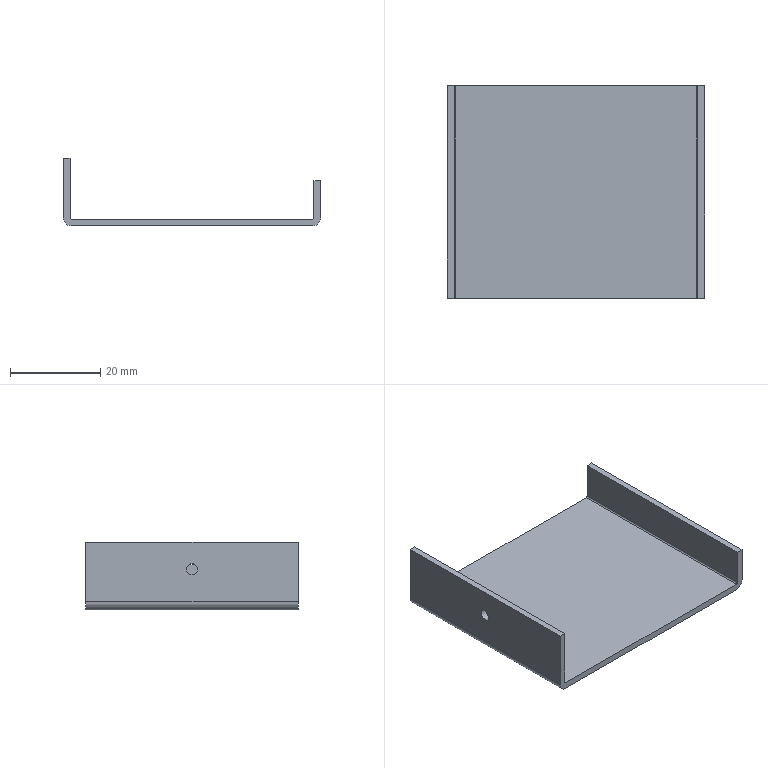Part | STEP file | FHD-021-008-01-B circuit breaker bracket 2 | 1 solid | 15 faces | box 57 x 47 x 15 mm | volume 5499 mm3 | plane 10 | cylinder 5 | commonest cylinder face diameters 0.6 x2 3.6 x2 2.5 x1
STEP:
#1=CARTESIAN_POINT('',(0.,0.,0.));
#2=DIRECTION('',(0.,0.,1.));
#3=DIRECTION('',(1.,0.,0.));
#4=AXIS2_PLACEMENT_3D('',#1,#2,#3);
#5=CARTESIAN_POINT('',(-26.7,23.5,-1.5));
#6=VERTEX_POINT('',#5);
#7=CARTESIAN_POINT('',(26.7,23.5,-1.5));
#8=VERTEX_POINT('',#7);
#9=CARTESIAN_POINT('',(0.,23.5,-1.5));
#10=DIRECTION('',(1.,0.,0.));
#11=VECTOR('',#10,1.);
#12=LINE('',#9,#11);
#13=CARTESIAN_POINT('',(0.,0.,-1.5));
#14=DIRECTION('',(0.,0.,-1.));
#15=DIRECTION('',(-1.,0.,0.));
#16=AXIS2_PLACEMENT_3D('',#13,#14,#15);
#17=PLANE('',#16);
#18=CARTESIAN_POINT('',(0.,23.5));
#19=DIRECTION('',(-1.,0.));
#20=VECTOR('',#19,1.);
#21=LINE('',#18,#20);
#22=(GEOMETRIC_REPRESENTATION_CONTEXT(2)PARAMETRIC_REPRESENTATION_CONTEXT()REPRESENTATION_CONTEXT('',''));
#23=DEFINITIONAL_REPRESENTATION('',(#21),#22);
#24=PCURVE('',#17,#23);
#25=CARTESIAN_POINT('',(-28.5,23.5,-1.5));
#26=DIRECTION('',(0.,1.,0.));
#27=DIRECTION('',(0.,0.,1.));
#28=AXIS2_PLACEMENT_3D('',#25,#26,#27);
#29=PLANE('',#28);
#30=CARTESIAN_POINT('',(0.,28.5));
#31=DIRECTION('',(0.,1.));
#32=VECTOR('',#31,1.);
#33=LINE('',#30,#32);
#34=(GEOMETRIC_REPRESENTATION_CONTEXT(2)PARAMETRIC_REPRESENTATION_CONTEXT()REPRESENTATION_CONTEXT('',''));
#35=DEFINITIONAL_REPRESENTATION('',(#33),#34);
#36=PCURVE('',#29,#35);
#37=SURFACE_CURVE('',#12,(#24,#36),.PCURVE_S1.);
#38=EDGE_CURVE('',#6,#8,#37,.T.);
#39=ORIENTED_EDGE('',*,*,#38,.T.);
#40=CARTESIAN_POINT('',(26.7,-23.5,-1.5));
#41=VERTEX_POINT('',#40);
#42=CARTESIAN_POINT('',(26.7,0.,-1.5));
#43=DIRECTION('',(0.,-1.,0.));
#44=VECTOR('',#43,1.);
#45=LINE('',#42,#44);
#46=CARTESIAN_POINT('',(-26.7,0.));
#47=DIRECTION('',(0.,-1.));
#48=VECTOR('',#47,1.);
#49=LINE('',#46,#48);
#50=(GEOMETRIC_REPRESENTATION_CONTEXT(2)PARAMETRIC_REPRESENTATION_CONTEXT()REPRESENTATION_CONTEXT('',''));
#51=DEFINITIONAL_REPRESENTATION('',(#49),#50);
#52=PCURVE('',#17,#51);
#53=CARTESIAN_POINT('',(26.7,23.5,0.3));
#54=DIRECTION('',(0.,1.,0.));
#55=DIRECTION('',(0.,0.,1.));
#56=AXIS2_PLACEMENT_3D('',#53,#54,#55);
#57=CYLINDRICAL_SURFACE('',#56,1.8);
#58=CARTESIAN_POINT('',(3.142,-23.5));
#59=DIRECTION('',(0.,-1.));
#60=VECTOR('',#59,1.);
#61=LINE('',#58,#60);
#62=(GEOMETRIC_REPRESENTATION_CONTEXT(2)PARAMETRIC_REPRESENTATION_CONTEXT()REPRESENTATION_CONTEXT('',''));
#63=DEFINITIONAL_REPRESENTATION('',(#61),#62);
#64=PCURVE('',#57,#63);
#65=SURFACE_CURVE('',#45,(#52,#64),.PCURVE_S1.);
#66=EDGE_CURVE('',#8,#41,#65,.T.);
#67=ORIENTED_EDGE('',*,*,#66,.T.);
#68=CARTESIAN_POINT('',(-26.7,-23.5,-1.5));
#69=VERTEX_POINT('',#68);
#70=CARTESIAN_POINT('',(0.,-23.5,-1.5));
#71=DIRECTION('',(-1.,0.,0.));
#72=VECTOR('',#71,1.);
#73=LINE('',#70,#72);
#74=CARTESIAN_POINT('',(0.,-23.5));
#75=DIRECTION('',(1.,0.));
#76=VECTOR('',#75,1.);
#77=LINE('',#74,#76);
#78=(GEOMETRIC_REPRESENTATION_CONTEXT(2)PARAMETRIC_REPRESENTATION_CONTEXT()REPRESENTATION_CONTEXT('',''));
#79=DEFINITIONAL_REPRESENTATION('',(#77),#78);
#80=PCURVE('',#17,#79);
#81=CARTESIAN_POINT('',(-28.5,-23.5,-1.5));
#82=DIRECTION('',(0.,-1.,0.));
#83=DIRECTION('',(0.,0.,-1.));
#84=AXIS2_PLACEMENT_3D('',#81,#82,#83);
#85=PLANE('',#84);
#86=CARTESIAN_POINT('',(0.,28.5));
#87=DIRECTION('',(0.,-1.));
#88=VECTOR('',#87,1.);
#89=LINE('',#86,#88);
#90=(GEOMETRIC_REPRESENTATION_CONTEXT(2)PARAMETRIC_REPRESENTATION_CONTEXT()REPRESENTATION_CONTEXT('',''));
#91=DEFINITIONAL_REPRESENTATION('',(#89),#90);
#92=PCURVE('',#85,#91);
#93=SURFACE_CURVE('',#73,(#80,#92),.PCURVE_S1.);
#94=EDGE_CURVE('',#41,#69,#93,.T.);
#95=ORIENTED_EDGE('',*,*,#94,.T.);
#96=CARTESIAN_POINT('',(-26.7,0.,-1.5));
#97=DIRECTION('',(0.,1.,0.));
#98=VECTOR('',#97,1.);
#99=LINE('',#96,#98);
#100=CARTESIAN_POINT('',(26.7,0.));
#101=DIRECTION('',(0.,1.));
#102=VECTOR('',#101,1.);
#103=LINE('',#100,#102);
#104=(GEOMETRIC_REPRESENTATION_CONTEXT(2)PARAMETRIC_REPRESENTATION_CONTEXT()REPRESENTATION_CONTEXT('',''));
#105=DEFINITIONAL_REPRESENTATION('',(#103),#104);
#106=PCURVE('',#17,#105);
#107=CARTESIAN_POINT('',(-26.7,-23.5,0.3));
#108=DIRECTION('',(0.,-1.,0.));
#109=DIRECTION('',(0.,0.,-1.));
#110=AXIS2_PLACEMENT_3D('',#107,#108,#109);
#111=CYLINDRICAL_SURFACE('',#110,1.8);
#112=CARTESIAN_POINT('',(6.283,-23.5));
#113=DIRECTION('',(0.,-1.));
#114=VECTOR('',#113,1.);
#115=LINE('',#112,#114);
#116=(GEOMETRIC_REPRESENTATION_CONTEXT(2)PARAMETRIC_REPRESENTATION_CONTEXT()REPRESENTATION_CONTEXT('',''));
#117=DEFINITIONAL_REPRESENTATION('',(#115),#116);
#118=PCURVE('',#111,#117);
#119=SURFACE_CURVE('',#99,(#106,#118),.PCURVE_S1.);
#120=EDGE_CURVE('',#69,#6,#119,.T.);
#121=ORIENTED_EDGE('',*,*,#120,.T.);
#122=EDGE_LOOP('',(#39,#67,#95,#121));
#123=FACE_BOUND('',#122,.T.);
#124=ADVANCED_FACE('',(#123),#17,.T.);
#125=CARTESIAN_POINT('',(28.5,23.5,0.3));
#126=VERTEX_POINT('',#125);
#127=CARTESIAN_POINT('',(28.5,-23.5,0.3));
#128=VERTEX_POINT('',#127);
#129=CARTESIAN_POINT('',(28.5,23.5,0.3));
#130=DIRECTION('',(0.,-1.,0.));
#131=VECTOR('',#130,1.);
#132=LINE('',#129,#131);
#133=CARTESIAN_POINT('',(1.571,0.));
#134=DIRECTION('',(0.,-1.));
#135=VECTOR('',#134,1.);
#136=LINE('',#133,#135);
#137=(GEOMETRIC_REPRESENTATION_CONTEXT(2)PARAMETRIC_REPRESENTATION_CONTEXT()REPRESENTATION_CONTEXT('',''));
#138=DEFINITIONAL_REPRESENTATION('',(#136),#137);
#139=PCURVE('',#57,#138);
#140=CARTESIAN_POINT('',(28.5,0.,0.));
#141=DIRECTION('',(-1.,0.,0.));
#142=DIRECTION('',(0.,0.,1.));
#143=AXIS2_PLACEMENT_3D('',#140,#141,#142);
#144=PLANE('',#143);
#145=CARTESIAN_POINT('',(0.3,23.5));
#146=DIRECTION('',(0.,-1.));
#147=VECTOR('',#146,1.);
#148=LINE('',#145,#147);
#149=(GEOMETRIC_REPRESENTATION_CONTEXT(2)PARAMETRIC_REPRESENTATION_CONTEXT()REPRESENTATION_CONTEXT('',''));
#150=DEFINITIONAL_REPRESENTATION('',(#148),#149);
#151=PCURVE('',#144,#150);
#152=SURFACE_CURVE('',#132,(#139,#151),.PCURVE_S1.);
#153=EDGE_CURVE('',#126,#128,#152,.T.);
#154=ORIENTED_EDGE('',*,*,#153,.T.);
#155=CARTESIAN_POINT('',(26.7,-23.5,0.3));
#156=DIRECTION('',(0.,1.,0.));
#157=DIRECTION('',(0.,0.,1.));
#158=AXIS2_PLACEMENT_3D('',#155,#156,#157);
#159=CIRCLE('',#158,1.8);
#160=CARTESIAN_POINT('',(0.,-47.));
#161=DIRECTION('',(1.,0.));
#162=VECTOR('',#161,1.);
#163=LINE('',#160,#162);
#164=(GEOMETRIC_REPRESENTATION_CONTEXT(2)PARAMETRIC_REPRESENTATION_CONTEXT()REPRESENTATION_CONTEXT('',''));
#165=DEFINITIONAL_REPRESENTATION('',(#163),#164);
#166=PCURVE('',#57,#165);
#167=CARTESIAN_POINT('',(-3.6,55.2));
#168=CARTESIAN_POINT('',(-3.6,58.318));
#169=CARTESIAN_POINT('',(-0.9,56.759));
#170=CARTESIAN_POINT('',(1.8,55.2));
#171=CARTESIAN_POINT('',(-0.9,53.641));
#172=CARTESIAN_POINT('',(-3.6,52.082));
#173=CARTESIAN_POINT('',(-3.6,55.2));
#174=(BOUNDED_CURVE()B_SPLINE_CURVE(2,(#167,#168,#169,#170,#171,#172,#173),.UNSPECIFIED.,.T.,.F.)B_SPLINE_CURVE_WITH_KNOTS((1,2,2,2,2,1),(-2.094,0.,2.094,4.189,6.283,8.378),.UNSPECIFIED.)CURVE()GEOMETRIC_REPRESENTATION_ITEM()RATIONAL_B_SPLINE_CURVE((1.,0.5,1.,0.5,1.,0.5,1.))REPRESENTATION_ITEM(''));
#175=(GEOMETRIC_REPRESENTATION_CONTEXT(2)PARAMETRIC_REPRESENTATION_CONTEXT()REPRESENTATION_CONTEXT('',''));
#176=DEFINITIONAL_REPRESENTATION('',(#174),#175);
#177=PCURVE('',#85,#176);
#178=SURFACE_CURVE('',#159,(#166,#177),.PCURVE_S1.);
#179=EDGE_CURVE('',#128,#41,#178,.T.);
#180=ORIENTED_EDGE('',*,*,#179,.T.);
#181=ORIENTED_EDGE('',*,*,#66,.F.);
#182=CARTESIAN_POINT('',(26.7,23.5,0.3));
#183=DIRECTION('',(0.,-1.,0.));
#184=DIRECTION('',(0.,0.,1.));
#185=AXIS2_PLACEMENT_3D('',#182,#183,#184);
#186=CIRCLE('',#185,1.8);
#187=CARTESIAN_POINT('',(6.283,0.));
#188=DIRECTION('',(-1.,0.));
#189=VECTOR('',#188,1.);
#190=LINE('',#187,#189);
#191=(GEOMETRIC_REPRESENTATION_CONTEXT(2)PARAMETRIC_REPRESENTATION_CONTEXT()REPRESENTATION_CONTEXT('',''));
#192=DEFINITIONAL_REPRESENTATION('',(#190),#191);
#193=PCURVE('',#57,#192);
#194=CARTESIAN_POINT('',(3.6,55.2));
#195=CARTESIAN_POINT('',(3.6,52.082));
#196=CARTESIAN_POINT('',(0.9,53.641));
#197=CARTESIAN_POINT('',(-1.8,55.2));
#198=CARTESIAN_POINT('',(0.9,56.759));
#199=CARTESIAN_POINT('',(3.6,58.318));
#200=CARTESIAN_POINT('',(3.6,55.2));
#201=(BOUNDED_CURVE()B_SPLINE_CURVE(2,(#194,#195,#196,#197,#198,#199,#200),.UNSPECIFIED.,.T.,.F.)B_SPLINE_CURVE_WITH_KNOTS((1,2,2,2,2,1),(-2.094,0.,2.094,4.189,6.283,8.378),.UNSPECIFIED.)CURVE()GEOMETRIC_REPRESENTATION_ITEM()RATIONAL_B_SPLINE_CURVE((1.,0.5,1.,0.5,1.,0.5,1.))REPRESENTATION_ITEM(''));
#202=(GEOMETRIC_REPRESENTATION_CONTEXT(2)PARAMETRIC_REPRESENTATION_CONTEXT()REPRESENTATION_CONTEXT('',''));
#203=DEFINITIONAL_REPRESENTATION('',(#201),#202);
#204=PCURVE('',#29,#203);
#205=SURFACE_CURVE('',#186,(#193,#204),.PCURVE_S1.);
#206=EDGE_CURVE('',#8,#126,#205,.T.);
#207=ORIENTED_EDGE('',*,*,#206,.T.);
#208=EDGE_LOOP('',(#154,#180,#181,#207));
#209=FACE_BOUND('',#208,.T.);
#210=ADVANCED_FACE('',(#209),#57,.T.);
#211=CARTESIAN_POINT('',(-26.7,23.5,0.));
#212=VERTEX_POINT('',#211);
#213=CARTESIAN_POINT('',(26.7,23.5,0.));
#214=VERTEX_POINT('',#213);
#215=CARTESIAN_POINT('',(-28.5,23.5,0.));
#216=DIRECTION('',(1.,0.,0.));
#217=VECTOR('',#216,1.);
#218=LINE('',#215,#217);
#219=CARTESIAN_POINT('',(1.5,0.));
#220=DIRECTION('',(0.,1.));
#221=VECTOR('',#220,1.);
#222=LINE('',#219,#221);
#223=(GEOMETRIC_REPRESENTATION_CONTEXT(2)PARAMETRIC_REPRESENTATION_CONTEXT()REPRESENTATION_CONTEXT('',''));
#224=DEFINITIONAL_REPRESENTATION('',(#222),#223);
#225=PCURVE('',#29,#224);
#226=CARTESIAN_POINT('',(0.,0.,0.));
#227=DIRECTION('',(0.,0.,-1.));
#228=DIRECTION('',(-1.,0.,0.));
#229=AXIS2_PLACEMENT_3D('',#226,#227,#228);
#230=PLANE('',#229);
#231=CARTESIAN_POINT('',(28.5,23.5));
#232=DIRECTION('',(-1.,0.));
#233=VECTOR('',#232,1.);
#234=LINE('',#231,#233);
#235=(GEOMETRIC_REPRESENTATION_CONTEXT(2)PARAMETRIC_REPRESENTATION_CONTEXT()REPRESENTATION_CONTEXT('',''));
#236=DEFINITIONAL_REPRESENTATION('',(#234),#235);
#237=PCURVE('',#230,#236);
#238=SURFACE_CURVE('',#218,(#225,#237),.PCURVE_S1.);
#239=EDGE_CURVE('',#212,#214,#238,.T.);
#240=ORIENTED_EDGE('',*,*,#239,.T.);
#241=CARTESIAN_POINT('',(27.,23.5,0.3));
#242=VERTEX_POINT('',#241);
#243=CARTESIAN_POINT('',(26.7,23.5,0.3));
#244=DIRECTION('',(0.,-1.,0.));
#245=DIRECTION('',(0.,0.,1.));
#246=AXIS2_PLACEMENT_3D('',#243,#244,#245);
#247=CIRCLE('',#246,0.3);
#248=CARTESIAN_POINT('',(2.1,55.2));
#249=CARTESIAN_POINT('',(2.1,54.68));
#250=CARTESIAN_POINT('',(1.65,54.94));
#251=CARTESIAN_POINT('',(1.2,55.2));
#252=CARTESIAN_POINT('',(1.65,55.46));
#253=CARTESIAN_POINT('',(2.1,55.72));
#254=CARTESIAN_POINT('',(2.1,55.2));
#255=(BOUNDED_CURVE()B_SPLINE_CURVE(2,(#248,#249,#250,#251,#252,#253,#254),.UNSPECIFIED.,.T.,.F.)B_SPLINE_CURVE_WITH_KNOTS((1,2,2,2,2,1),(-2.094,0.,2.094,4.189,6.283,8.378),.UNSPECIFIED.)CURVE()GEOMETRIC_REPRESENTATION_ITEM()RATIONAL_B_SPLINE_CURVE((1.,0.5,1.,0.5,1.,0.5,1.))REPRESENTATION_ITEM(''));
#256=(GEOMETRIC_REPRESENTATION_CONTEXT(2)PARAMETRIC_REPRESENTATION_CONTEXT()REPRESENTATION_CONTEXT('',''));
#257=DEFINITIONAL_REPRESENTATION('',(#255),#256);
#258=PCURVE('',#29,#257);
#259=CARTESIAN_POINT('',(26.7,23.5,0.3));
#260=DIRECTION('',(0.,1.,0.));
#261=DIRECTION('',(0.,0.,1.));
#262=AXIS2_PLACEMENT_3D('',#259,#260,#261);
#263=CYLINDRICAL_SURFACE('',#262,0.3);
#264=CARTESIAN_POINT('',(6.283,0.));
#265=DIRECTION('',(-1.,0.));
#266=VECTOR('',#265,1.);
#267=LINE('',#264,#266);
#268=(GEOMETRIC_REPRESENTATION_CONTEXT(2)PARAMETRIC_REPRESENTATION_CONTEXT()REPRESENTATION_CONTEXT('',''));
#269=DEFINITIONAL_REPRESENTATION('',(#267),#268);
#270=PCURVE('',#263,#269);
#271=SURFACE_CURVE('',#247,(#258,#270),.PCURVE_S1.);
#272=EDGE_CURVE('',#214,#242,#271,.T.);
#273=ORIENTED_EDGE('',*,*,#272,.T.);
#274=CARTESIAN_POINT('',(27.,23.5,8.5));
#275=VERTEX_POINT('',#274);
#276=CARTESIAN_POINT('',(27.,23.5,13.5));
#277=DIRECTION('',(0.,0.,-1.));
#278=VECTOR('',#277,1.);
#279=LINE('',#276,#278);
#280=CARTESIAN_POINT('',(15.,55.5));
#281=DIRECTION('',(-1.,0.));
#282=VECTOR('',#281,1.);
#283=LINE('',#280,#282);
#284=(GEOMETRIC_REPRESENTATION_CONTEXT(2)PARAMETRIC_REPRESENTATION_CONTEXT()REPRESENTATION_CONTEXT('',''));
#285=DEFINITIONAL_REPRESENTATION('',(#283),#284);
#286=PCURVE('',#29,#285);
#287=CARTESIAN_POINT('',(27.,0.,0.));
#288=DIRECTION('',(-1.,0.,0.));
#289=DIRECTION('',(0.,0.,1.));
#290=AXIS2_PLACEMENT_3D('',#287,#288,#289);
#291=PLANE('',#290);
#292=CARTESIAN_POINT('',(13.5,23.5));
#293=DIRECTION('',(-1.,0.));
#294=VECTOR('',#293,1.);
#295=LINE('',#292,#294);
#296=(GEOMETRIC_REPRESENTATION_CONTEXT(2)PARAMETRIC_REPRESENTATION_CONTEXT()REPRESENTATION_CONTEXT('',''));
#297=DEFINITIONAL_REPRESENTATION('',(#295),#296);
#298=PCURVE('',#291,#297);
#299=SURFACE_CURVE('',#279,(#286,#298),.PCURVE_S1.);
#300=EDGE_CURVE('',#275,#242,#299,.T.);
#301=ORIENTED_EDGE('',*,*,#300,.F.);
#302=CARTESIAN_POINT('',(28.5,23.5,8.5));
#303=VERTEX_POINT('',#302);
#304=CARTESIAN_POINT('',(28.5,23.5,8.5));
#305=DIRECTION('',(-1.,0.,0.));
#306=VECTOR('',#305,1.);
#307=LINE('',#304,#306);
#308=CARTESIAN_POINT('',(10.,57.));
#309=DIRECTION('',(0.,-1.));
#310=VECTOR('',#309,1.);
#311=LINE('',#308,#310);
#312=(GEOMETRIC_REPRESENTATION_CONTEXT(2)PARAMETRIC_REPRESENTATION_CONTEXT()REPRESENTATION_CONTEXT('',''));
#313=DEFINITIONAL_REPRESENTATION('',(#311),#312);
#314=PCURVE('',#29,#313);
#315=CARTESIAN_POINT('',(37.,23.5,8.5));
#316=DIRECTION('',(0.,0.,-1.));
#317=DIRECTION('',(-1.,0.,0.));
#318=AXIS2_PLACEMENT_3D('',#315,#316,#317);
#319=PLANE('',#318);
#320=CARTESIAN_POINT('',(8.5,0.));
#321=DIRECTION('',(1.,0.));
#322=VECTOR('',#321,1.);
#323=LINE('',#320,#322);
#324=(GEOMETRIC_REPRESENTATION_CONTEXT(2)PARAMETRIC_REPRESENTATION_CONTEXT()REPRESENTATION_CONTEXT('',''));
#325=DEFINITIONAL_REPRESENTATION('',(#323),#324);
#326=PCURVE('',#319,#325);
#327=SURFACE_CURVE('',#307,(#314,#326),.PCURVE_S1.);
#328=EDGE_CURVE('',#303,#275,#327,.T.);
#329=ORIENTED_EDGE('',*,*,#328,.F.);
#330=CARTESIAN_POINT('',(28.5,23.5,0.));
#331=DIRECTION('',(0.,0.,-1.));
#332=VECTOR('',#331,1.);
#333=LINE('',#330,#332);
#334=CARTESIAN_POINT('',(1.5,57.));
#335=DIRECTION('',(-1.,0.));
#336=VECTOR('',#335,1.);
#337=LINE('',#334,#336);
#338=(GEOMETRIC_REPRESENTATION_CONTEXT(2)PARAMETRIC_REPRESENTATION_CONTEXT()REPRESENTATION_CONTEXT('',''));
#339=DEFINITIONAL_REPRESENTATION('',(#337),#338);
#340=PCURVE('',#29,#339);
#341=CARTESIAN_POINT('',(0.,23.5));
#342=DIRECTION('',(-1.,0.));
#343=VECTOR('',#342,1.);
#344=LINE('',#341,#343);
#345=(GEOMETRIC_REPRESENTATION_CONTEXT(2)PARAMETRIC_REPRESENTATION_CONTEXT()REPRESENTATION_CONTEXT('',''));
#346=DEFINITIONAL_REPRESENTATION('',(#344),#345);
#347=PCURVE('',#144,#346);
#348=SURFACE_CURVE('',#333,(#340,#347),.PCURVE_S1.);
#349=EDGE_CURVE('',#303,#126,#348,.T.);
#350=ORIENTED_EDGE('',*,*,#349,.T.);
#351=ORIENTED_EDGE('',*,*,#206,.F.);
#352=ORIENTED_EDGE('',*,*,#38,.F.);
#353=CARTESIAN_POINT('',(-28.5,23.5,0.3));
#354=VERTEX_POINT('',#353);
#355=CARTESIAN_POINT('',(-26.7,23.5,0.3));
#356=DIRECTION('',(0.,-1.,0.));
#357=DIRECTION('',(0.,0.,-1.));
#358=AXIS2_PLACEMENT_3D('',#355,#356,#357);
#359=CIRCLE('',#358,1.8);
#360=CARTESIAN_POINT('',(0.,1.8));
#361=CARTESIAN_POINT('',(0.,4.918));
#362=CARTESIAN_POINT('',(2.7,3.359));
#363=CARTESIAN_POINT('',(5.4,1.8));
#364=CARTESIAN_POINT('',(2.7,0.2412));
#365=CARTESIAN_POINT('',(0.,-1.318));
#366=CARTESIAN_POINT('',(0.,1.8));
#367=(BOUNDED_CURVE()B_SPLINE_CURVE(2,(#360,#361,#362,#363,#364,#365,#366),.UNSPECIFIED.,.T.,.F.)B_SPLINE_CURVE_WITH_KNOTS((1,2,2,2,2,1),(-2.094,0.,2.094,4.189,6.283,8.378),.UNSPECIFIED.)CURVE()GEOMETRIC_REPRESENTATION_ITEM()RATIONAL_B_SPLINE_CURVE((1.,0.5,1.,0.5,1.,0.5,1.))REPRESENTATION_ITEM(''));
#368=(GEOMETRIC_REPRESENTATION_CONTEXT(2)PARAMETRIC_REPRESENTATION_CONTEXT()REPRESENTATION_CONTEXT('',''));
#369=DEFINITIONAL_REPRESENTATION('',(#367),#368);
#370=PCURVE('',#29,#369);
#371=CARTESIAN_POINT('',(0.,-47.));
#372=DIRECTION('',(1.,0.));
#373=VECTOR('',#372,1.);
#374=LINE('',#371,#373);
#375=(GEOMETRIC_REPRESENTATION_CONTEXT(2)PARAMETRIC_REPRESENTATION_CONTEXT()REPRESENTATION_CONTEXT('',''));
#376=DEFINITIONAL_REPRESENTATION('',(#374),#375);
#377=PCURVE('',#111,#376);
#378=SURFACE_CURVE('',#359,(#370,#377),.PCURVE_S1.);
#379=EDGE_CURVE('',#354,#6,#378,.T.);
#380=ORIENTED_EDGE('',*,*,#379,.F.);
#381=CARTESIAN_POINT('',(-28.5,23.5,13.5));
#382=VERTEX_POINT('',#381);
#383=CARTESIAN_POINT('',(-28.5,23.5,0.));
#384=DIRECTION('',(0.,0.,1.));
#385=VECTOR('',#384,1.);
#386=LINE('',#383,#385);
#387=CARTESIAN_POINT('',(1.5,0.));
#388=DIRECTION('',(1.,0.));
#389=VECTOR('',#388,1.);
#390=LINE('',#387,#389);
#391=(GEOMETRIC_REPRESENTATION_CONTEXT(2)PARAMETRIC_REPRESENTATION_CONTEXT()REPRESENTATION_CONTEXT('',''));
#392=DEFINITIONAL_REPRESENTATION('',(#390),#391);
#393=PCURVE('',#29,#392);
#394=CARTESIAN_POINT('',(-28.5,0.,0.));
#395=DIRECTION('',(1.,0.,0.));
#396=DIRECTION('',(0.,0.,-1.));
#397=AXIS2_PLACEMENT_3D('',#394,#395,#396);
#398=PLANE('',#397);
#399=CARTESIAN_POINT('',(0.,23.5));
#400=DIRECTION('',(-1.,0.));
#401=VECTOR('',#400,1.);
#402=LINE('',#399,#401);
#403=(GEOMETRIC_REPRESENTATION_CONTEXT(2)PARAMETRIC_REPRESENTATION_CONTEXT()REPRESENTATION_CONTEXT('',''));
#404=DEFINITIONAL_REPRESENTATION('',(#402),#403);
#405=PCURVE('',#398,#404);
#406=SURFACE_CURVE('',#386,(#393,#405),.PCURVE_S1.);
#407=EDGE_CURVE('',#354,#382,#406,.T.);
#408=ORIENTED_EDGE('',*,*,#407,.T.);
#409=CARTESIAN_POINT('',(-27.,23.5,13.5));
#410=VERTEX_POINT('',#409);
#411=CARTESIAN_POINT('',(-28.5,23.5,13.5));
#412=DIRECTION('',(1.,0.,0.));
#413=VECTOR('',#412,1.);
#414=LINE('',#411,#413);
#415=CARTESIAN_POINT('',(15.,0.));
#416=DIRECTION('',(0.,1.));
#417=VECTOR('',#416,1.);
#418=LINE('',#415,#417);
#419=(GEOMETRIC_REPRESENTATION_CONTEXT(2)PARAMETRIC_REPRESENTATION_CONTEXT()REPRESENTATION_CONTEXT('',''));
#420=DEFINITIONAL_REPRESENTATION('',(#418),#419);
#421=PCURVE('',#29,#420);
#422=CARTESIAN_POINT('',(-28.5,23.5,13.5));
#423=DIRECTION('',(0.,0.,-1.));
#424=DIRECTION('',(-1.,0.,0.));
#425=AXIS2_PLACEMENT_3D('',#422,#423,#424);
#426=PLANE('',#425);
#427=CARTESIAN_POINT('',(0.,0.));
#428=DIRECTION('',(-1.,0.));
#429=VECTOR('',#428,1.);
#430=LINE('',#427,#429);
#431=(GEOMETRIC_REPRESENTATION_CONTEXT(2)PARAMETRIC_REPRESENTATION_CONTEXT()REPRESENTATION_CONTEXT('',''));
#432=DEFINITIONAL_REPRESENTATION('',(#430),#431);
#433=PCURVE('',#426,#432);
#434=SURFACE_CURVE('',#414,(#421,#433),.PCURVE_S1.);
#435=EDGE_CURVE('',#382,#410,#434,.T.);
#436=ORIENTED_EDGE('',*,*,#435,.T.);
#437=CARTESIAN_POINT('',(-27.,23.5,0.3));
#438=VERTEX_POINT('',#437);
#439=CARTESIAN_POINT('',(-27.,23.5,0.));
#440=DIRECTION('',(0.,0.,1.));
#441=VECTOR('',#440,1.);
#442=LINE('',#439,#441);
#443=CARTESIAN_POINT('',(1.5,1.5));
#444=DIRECTION('',(1.,0.));
#445=VECTOR('',#444,1.);
#446=LINE('',#443,#445);
#447=(GEOMETRIC_REPRESENTATION_CONTEXT(2)PARAMETRIC_REPRESENTATION_CONTEXT()REPRESENTATION_CONTEXT('',''));
#448=DEFINITIONAL_REPRESENTATION('',(#446),#447);
#449=PCURVE('',#29,#448);
#450=CARTESIAN_POINT('',(-27.,0.,0.));
#451=DIRECTION('',(1.,0.,0.));
#452=DIRECTION('',(0.,0.,-1.));
#453=AXIS2_PLACEMENT_3D('',#450,#451,#452);
#454=PLANE('',#453);
#455=CARTESIAN_POINT('',(0.,23.5));
#456=DIRECTION('',(-1.,0.));
#457=VECTOR('',#456,1.);
#458=LINE('',#455,#457);
#459=(GEOMETRIC_REPRESENTATION_CONTEXT(2)PARAMETRIC_REPRESENTATION_CONTEXT()REPRESENTATION_CONTEXT('',''));
#460=DEFINITIONAL_REPRESENTATION('',(#458),#459);
#461=PCURVE('',#454,#460);
#462=SURFACE_CURVE('',#442,(#449,#461),.PCURVE_S1.);
#463=EDGE_CURVE('',#438,#410,#462,.T.);
#464=ORIENTED_EDGE('',*,*,#463,.F.);
#465=CARTESIAN_POINT('',(-26.7,23.5,0.3));
#466=DIRECTION('',(0.,-1.,0.));
#467=DIRECTION('',(0.,0.,-1.));
#468=AXIS2_PLACEMENT_3D('',#465,#466,#467);
#469=CIRCLE('',#468,0.3);
#470=CARTESIAN_POINT('',(1.5,1.8));
#471=CARTESIAN_POINT('',(1.5,2.32));
#472=CARTESIAN_POINT('',(1.95,2.06));
#473=CARTESIAN_POINT('',(2.4,1.8));
#474=CARTESIAN_POINT('',(1.95,1.54));
#475=CARTESIAN_POINT('',(1.5,1.28));
#476=CARTESIAN_POINT('',(1.5,1.8));
#477=(BOUNDED_CURVE()B_SPLINE_CURVE(2,(#470,#471,#472,#473,#474,#475,#476),.UNSPECIFIED.,.T.,.F.)B_SPLINE_CURVE_WITH_KNOTS((1,2,2,2,2,1),(-2.094,0.,2.094,4.189,6.283,8.378),.UNSPECIFIED.)CURVE()GEOMETRIC_REPRESENTATION_ITEM()RATIONAL_B_SPLINE_CURVE((1.,0.5,1.,0.5,1.,0.5,1.))REPRESENTATION_ITEM(''));
#478=(GEOMETRIC_REPRESENTATION_CONTEXT(2)PARAMETRIC_REPRESENTATION_CONTEXT()REPRESENTATION_CONTEXT('',''));
#479=DEFINITIONAL_REPRESENTATION('',(#477),#478);
#480=PCURVE('',#29,#479);
#481=CARTESIAN_POINT('',(-26.7,-23.5,0.3));
#482=DIRECTION('',(0.,-1.,0.));
#483=DIRECTION('',(0.,0.,-1.));
#484=AXIS2_PLACEMENT_3D('',#481,#482,#483);
#485=CYLINDRICAL_SURFACE('',#484,0.3);
#486=CARTESIAN_POINT('',(0.,-47.));
#487=DIRECTION('',(1.,0.));
#488=VECTOR('',#487,1.);
#489=LINE('',#486,#488);
#490=(GEOMETRIC_REPRESENTATION_CONTEXT(2)PARAMETRIC_REPRESENTATION_CONTEXT()REPRESENTATION_CONTEXT('',''));
#491=DEFINITIONAL_REPRESENTATION('',(#489),#490);
#492=PCURVE('',#485,#491);
#493=SURFACE_CURVE('',#469,(#480,#492),.PCURVE_S1.);
#494=EDGE_CURVE('',#438,#212,#493,.T.);
#495=ORIENTED_EDGE('',*,*,#494,.T.);
#496=EDGE_LOOP('',(#240,#273,#301,#329,#350,#351,#352,#380,#408,#436,#464,#495));
#497=FACE_BOUND('',#496,.T.);
#498=ADVANCED_FACE('',(#497),#29,.T.);
#499=CARTESIAN_POINT('',(-28.5,-23.5,0.3));
#500=VERTEX_POINT('',#499);
#501=CARTESIAN_POINT('',(-28.5,-23.5,0.3));
#502=DIRECTION('',(0.,1.,0.));
#503=VECTOR('',#502,1.);
#504=LINE('',#501,#503);
#505=CARTESIAN_POINT('',(4.712,0.));
#506=DIRECTION('',(0.,-1.));
#507=VECTOR('',#506,1.);
#508=LINE('',#505,#507);
#509=(GEOMETRIC_REPRESENTATION_CONTEXT(2)PARAMETRIC_REPRESENTATION_CONTEXT()REPRESENTATION_CONTEXT('',''));
#510=DEFINITIONAL_REPRESENTATION('',(#508),#509);
#511=PCURVE('',#111,#510);
#512=CARTESIAN_POINT('',(-0.3,-23.5));
#513=DIRECTION('',(0.,1.));
#514=VECTOR('',#513,1.);
#515=LINE('',#512,#514);
#516=(GEOMETRIC_REPRESENTATION_CONTEXT(2)PARAMETRIC_REPRESENTATION_CONTEXT()REPRESENTATION_CONTEXT('',''));
#517=DEFINITIONAL_REPRESENTATION('',(#515),#516);
#518=PCURVE('',#398,#517);
#519=SURFACE_CURVE('',#504,(#511,#518),.PCURVE_S1.);
#520=EDGE_CURVE('',#500,#354,#519,.T.);
#521=ORIENTED_EDGE('',*,*,#520,.T.);
#522=ORIENTED_EDGE('',*,*,#379,.T.);
#523=ORIENTED_EDGE('',*,*,#120,.F.);
#524=CARTESIAN_POINT('',(-26.7,-23.5,0.3));
#525=DIRECTION('',(0.,1.,0.));
#526=DIRECTION('',(0.,0.,-1.));
#527=AXIS2_PLACEMENT_3D('',#524,#525,#526);
#528=CIRCLE('',#527,1.8);
#529=CARTESIAN_POINT('',(6.283,0.));
#530=DIRECTION('',(-1.,0.));
#531=VECTOR('',#530,1.);
#532=LINE('',#529,#531);
#533=(GEOMETRIC_REPRESENTATION_CONTEXT(2)PARAMETRIC_REPRESENTATION_CONTEXT()REPRESENTATION_CONTEXT('',''));
#534=DEFINITIONAL_REPRESENTATION('',(#532),#533);
#535=PCURVE('',#111,#534);
#536=CARTESIAN_POINT('',(0.,1.8));
#537=CARTESIAN_POINT('',(0.,-1.318));
#538=CARTESIAN_POINT('',(-2.7,0.2412));
#539=CARTESIAN_POINT('',(-5.4,1.8));
#540=CARTESIAN_POINT('',(-2.7,3.359));
#541=CARTESIAN_POINT('',(0.,4.918));
#542=CARTESIAN_POINT('',(0.,1.8));
#543=(BOUNDED_CURVE()B_SPLINE_CURVE(2,(#536,#537,#538,#539,#540,#541,#542),.UNSPECIFIED.,.T.,.F.)B_SPLINE_CURVE_WITH_KNOTS((1,2,2,2,2,1),(-2.094,0.,2.094,4.189,6.283,8.378),.UNSPECIFIED.)CURVE()GEOMETRIC_REPRESENTATION_ITEM()RATIONAL_B_SPLINE_CURVE((1.,0.5,1.,0.5,1.,0.5,1.))REPRESENTATION_ITEM(''));
#544=(GEOMETRIC_REPRESENTATION_CONTEXT(2)PARAMETRIC_REPRESENTATION_CONTEXT()REPRESENTATION_CONTEXT('',''));
#545=DEFINITIONAL_REPRESENTATION('',(#543),#544);
#546=PCURVE('',#85,#545);
#547=SURFACE_CURVE('',#528,(#535,#546),.PCURVE_S1.);
#548=EDGE_CURVE('',#69,#500,#547,.T.);
#549=ORIENTED_EDGE('',*,*,#548,.T.);
#550=EDGE_LOOP('',(#521,#522,#523,#549));
#551=FACE_BOUND('',#550,.T.);
#552=ADVANCED_FACE('',(#551),#111,.T.);
#553=ORIENTED_EDGE('',*,*,#94,.F.);
#554=ORIENTED_EDGE('',*,*,#179,.F.);
#555=CARTESIAN_POINT('',(28.5,-23.5,8.5));
#556=VERTEX_POINT('',#555);
#557=CARTESIAN_POINT('',(28.5,-23.5,0.));
#558=DIRECTION('',(0.,0.,1.));
#559=VECTOR('',#558,1.);
#560=LINE('',#557,#559);
#561=CARTESIAN_POINT('',(-1.5,57.));
#562=DIRECTION('',(-1.,0.));
#563=VECTOR('',#562,1.);
#564=LINE('',#561,#563);
#565=(GEOMETRIC_REPRESENTATION_CONTEXT(2)PARAMETRIC_REPRESENTATION_CONTEXT()REPRESENTATION_CONTEXT('',''));
#566=DEFINITIONAL_REPRESENTATION('',(#564),#565);
#567=PCURVE('',#85,#566);
#568=CARTESIAN_POINT('',(0.,-23.5));
#569=DIRECTION('',(1.,0.));
#570=VECTOR('',#569,1.);
#571=LINE('',#568,#570);
#572=(GEOMETRIC_REPRESENTATION_CONTEXT(2)PARAMETRIC_REPRESENTATION_CONTEXT()REPRESENTATION_CONTEXT('',''));
#573=DEFINITIONAL_REPRESENTATION('',(#571),#572);
#574=PCURVE('',#144,#573);
#575=SURFACE_CURVE('',#560,(#567,#574),.PCURVE_S1.);
#576=EDGE_CURVE('',#128,#556,#575,.T.);
#577=ORIENTED_EDGE('',*,*,#576,.T.);
#578=CARTESIAN_POINT('',(27.,-23.5,8.5));
#579=VERTEX_POINT('',#578);
#580=CARTESIAN_POINT('',(37.,-23.5,8.5));
#581=DIRECTION('',(-1.,0.,0.));
#582=VECTOR('',#581,1.);
#583=LINE('',#580,#582);
#584=CARTESIAN_POINT('',(-10.,65.5));
#585=DIRECTION('',(0.,-1.));
#586=VECTOR('',#585,1.);
#587=LINE('',#584,#586);
#588=(GEOMETRIC_REPRESENTATION_CONTEXT(2)PARAMETRIC_REPRESENTATION_CONTEXT()REPRESENTATION_CONTEXT('',''));
#589=DEFINITIONAL_REPRESENTATION('',(#587),#588);
#590=PCURVE('',#85,#589);
#591=CARTESIAN_POINT('',(0.,-47.));
#592=DIRECTION('',(1.,0.));
#593=VECTOR('',#592,1.);
#594=LINE('',#591,#593);
#595=(GEOMETRIC_REPRESENTATION_CONTEXT(2)PARAMETRIC_REPRESENTATION_CONTEXT()REPRESENTATION_CONTEXT('',''));
#596=DEFINITIONAL_REPRESENTATION('',(#594),#595);
#597=PCURVE('',#319,#596);
#598=SURFACE_CURVE('',#583,(#590,#597),.PCURVE_S1.);
#599=EDGE_CURVE('',#556,#579,#598,.T.);
#600=ORIENTED_EDGE('',*,*,#599,.T.);
#601=CARTESIAN_POINT('',(27.,-23.5,0.3));
#602=VERTEX_POINT('',#601);
#603=CARTESIAN_POINT('',(27.,-23.5,0.));
#604=DIRECTION('',(0.,0.,1.));
#605=VECTOR('',#604,1.);
#606=LINE('',#603,#605);
#607=CARTESIAN_POINT('',(-1.5,55.5));
#608=DIRECTION('',(-1.,0.));
#609=VECTOR('',#608,1.);
#610=LINE('',#607,#609);
#611=(GEOMETRIC_REPRESENTATION_CONTEXT(2)PARAMETRIC_REPRESENTATION_CONTEXT()REPRESENTATION_CONTEXT('',''));
#612=DEFINITIONAL_REPRESENTATION('',(#610),#611);
#613=PCURVE('',#85,#612);
#614=CARTESIAN_POINT('',(0.,-23.5));
#615=DIRECTION('',(1.,0.));
#616=VECTOR('',#615,1.);
#617=LINE('',#614,#616);
#618=(GEOMETRIC_REPRESENTATION_CONTEXT(2)PARAMETRIC_REPRESENTATION_CONTEXT()REPRESENTATION_CONTEXT('',''));
#619=DEFINITIONAL_REPRESENTATION('',(#617),#618);
#620=PCURVE('',#291,#619);
#621=SURFACE_CURVE('',#606,(#613,#620),.PCURVE_S1.);
#622=EDGE_CURVE('',#602,#579,#621,.T.);
#623=ORIENTED_EDGE('',*,*,#622,.F.);
#624=CARTESIAN_POINT('',(26.7,-23.5,0.));
#625=VERTEX_POINT('',#624);
#626=CARTESIAN_POINT('',(26.7,-23.5,0.3));
#627=DIRECTION('',(0.,1.,0.));
#628=DIRECTION('',(0.,0.,1.));
#629=AXIS2_PLACEMENT_3D('',#626,#627,#628);
#630=CIRCLE('',#629,0.3);
#631=CARTESIAN_POINT('',(-2.1,55.2));
#632=CARTESIAN_POINT('',(-2.1,55.72));
#633=CARTESIAN_POINT('',(-1.65,55.46));
#634=CARTESIAN_POINT('',(-1.2,55.2));
#635=CARTESIAN_POINT('',(-1.65,54.94));
#636=CARTESIAN_POINT('',(-2.1,54.68));
#637=CARTESIAN_POINT('',(-2.1,55.2));
#638=(BOUNDED_CURVE()B_SPLINE_CURVE(2,(#631,#632,#633,#634,#635,#636,#637),.UNSPECIFIED.,.T.,.F.)B_SPLINE_CURVE_WITH_KNOTS((1,2,2,2,2,1),(-2.094,0.,2.094,4.189,6.283,8.378),.UNSPECIFIED.)CURVE()GEOMETRIC_REPRESENTATION_ITEM()RATIONAL_B_SPLINE_CURVE((1.,0.5,1.,0.5,1.,0.5,1.))REPRESENTATION_ITEM(''));
#639=(GEOMETRIC_REPRESENTATION_CONTEXT(2)PARAMETRIC_REPRESENTATION_CONTEXT()REPRESENTATION_CONTEXT('',''));
#640=DEFINITIONAL_REPRESENTATION('',(#638),#639);
#641=PCURVE('',#85,#640);
#642=CARTESIAN_POINT('',(0.,-47.));
#643=DIRECTION('',(1.,0.));
#644=VECTOR('',#643,1.);
#645=LINE('',#642,#644);
#646=(GEOMETRIC_REPRESENTATION_CONTEXT(2)PARAMETRIC_REPRESENTATION_CONTEXT()REPRESENTATION_CONTEXT('',''));
#647=DEFINITIONAL_REPRESENTATION('',(#645),#646);
#648=PCURVE('',#263,#647);
#649=SURFACE_CURVE('',#630,(#641,#648),.PCURVE_S1.);
#650=EDGE_CURVE('',#602,#625,#649,.T.);
#651=ORIENTED_EDGE('',*,*,#650,.T.);
#652=CARTESIAN_POINT('',(-26.7,-23.5,0.));
#653=VERTEX_POINT('',#652);
#654=CARTESIAN_POINT('',(-28.5,-23.5,0.));
#655=DIRECTION('',(-1.,0.,0.));
#656=VECTOR('',#655,1.);
#657=LINE('',#654,#656);
#658=CARTESIAN_POINT('',(-1.5,0.));
#659=DIRECTION('',(0.,-1.));
#660=VECTOR('',#659,1.);
#661=LINE('',#658,#660);
#662=(GEOMETRIC_REPRESENTATION_CONTEXT(2)PARAMETRIC_REPRESENTATION_CONTEXT()REPRESENTATION_CONTEXT('',''));
#663=DEFINITIONAL_REPRESENTATION('',(#661),#662);
#664=PCURVE('',#85,#663);
#665=CARTESIAN_POINT('',(28.5,-23.5));
#666=DIRECTION('',(1.,0.));
#667=VECTOR('',#666,1.);
#668=LINE('',#665,#667);
#669=(GEOMETRIC_REPRESENTATION_CONTEXT(2)PARAMETRIC_REPRESENTATION_CONTEXT()REPRESENTATION_CONTEXT('',''));
#670=DEFINITIONAL_REPRESENTATION('',(#668),#669);
#671=PCURVE('',#230,#670);
#672=SURFACE_CURVE('',#657,(#664,#671),.PCURVE_S1.);
#673=EDGE_CURVE('',#625,#653,#672,.T.);
#674=ORIENTED_EDGE('',*,*,#673,.T.);
#675=CARTESIAN_POINT('',(-27.,-23.5,0.3));
#676=VERTEX_POINT('',#675);
#677=CARTESIAN_POINT('',(-26.7,-23.5,0.3));
#678=DIRECTION('',(0.,-1.,0.));
#679=DIRECTION('',(0.,0.,-1.));
#680=AXIS2_PLACEMENT_3D('',#677,#678,#679);
#681=CIRCLE('',#680,0.3);
#682=CARTESIAN_POINT('',(-1.8,1.8));
#683=DIRECTION('',(1.,0.));
#684=AXIS2_PLACEMENT_2D('',#682,#683);
#685=CIRCLE('',#684,0.3);
#686=(GEOMETRIC_REPRESENTATION_CONTEXT(2)PARAMETRIC_REPRESENTATION_CONTEXT()REPRESENTATION_CONTEXT('',''));
#687=DEFINITIONAL_REPRESENTATION('',(#685),#686);
#688=PCURVE('',#85,#687);
#689=CARTESIAN_POINT('',(0.,0.));
#690=DIRECTION('',(1.,0.));
#691=VECTOR('',#690,1.);
#692=LINE('',#689,#691);
#693=(GEOMETRIC_REPRESENTATION_CONTEXT(2)PARAMETRIC_REPRESENTATION_CONTEXT()REPRESENTATION_CONTEXT('',''));
#694=DEFINITIONAL_REPRESENTATION('',(#692),#693);
#695=PCURVE('',#485,#694);
#696=SURFACE_CURVE('',#681,(#688,#695),.PCURVE_S1.);
#697=EDGE_CURVE('',#676,#653,#696,.T.);
#698=ORIENTED_EDGE('',*,*,#697,.F.);
#699=CARTESIAN_POINT('',(-27.,-23.5,13.5));
#700=VERTEX_POINT('',#699);
#701=CARTESIAN_POINT('',(-27.,-23.5,13.5));
#702=DIRECTION('',(0.,0.,-1.));
#703=VECTOR('',#702,1.);
#704=LINE('',#701,#703);
#705=CARTESIAN_POINT('',(-15.,1.5));
#706=DIRECTION('',(1.,0.));
#707=VECTOR('',#706,1.);
#708=LINE('',#705,#707);
#709=(GEOMETRIC_REPRESENTATION_CONTEXT(2)PARAMETRIC_REPRESENTATION_CONTEXT()REPRESENTATION_CONTEXT('',''));
#710=DEFINITIONAL_REPRESENTATION('',(#708),#709);
#711=PCURVE('',#85,#710);
#712=CARTESIAN_POINT('',(-13.5,-23.5));
#713=DIRECTION('',(1.,0.));
#714=VECTOR('',#713,1.);
#715=LINE('',#712,#714);
#716=(GEOMETRIC_REPRESENTATION_CONTEXT(2)PARAMETRIC_REPRESENTATION_CONTEXT()REPRESENTATION_CONTEXT('',''));
#717=DEFINITIONAL_REPRESENTATION('',(#715),#716);
#718=PCURVE('',#454,#717);
#719=SURFACE_CURVE('',#704,(#711,#718),.PCURVE_S1.);
#720=EDGE_CURVE('',#700,#676,#719,.T.);
#721=ORIENTED_EDGE('',*,*,#720,.F.);
#722=CARTESIAN_POINT('',(-28.5,-23.5,13.5));
#723=VERTEX_POINT('',#722);
#724=CARTESIAN_POINT('',(-28.5,-23.5,13.5));
#725=DIRECTION('',(1.,0.,0.));
#726=VECTOR('',#725,1.);
#727=LINE('',#724,#726);
#728=CARTESIAN_POINT('',(-15.,0.));
#729=DIRECTION('',(0.,1.));
#730=VECTOR('',#729,1.);
#731=LINE('',#728,#730);
#732=(GEOMETRIC_REPRESENTATION_CONTEXT(2)PARAMETRIC_REPRESENTATION_CONTEXT()REPRESENTATION_CONTEXT('',''));
#733=DEFINITIONAL_REPRESENTATION('',(#731),#732);
#734=PCURVE('',#85,#733);
#735=CARTESIAN_POINT('',(0.,-47.));
#736=DIRECTION('',(-1.,0.));
#737=VECTOR('',#736,1.);
#738=LINE('',#735,#737);
#739=(GEOMETRIC_REPRESENTATION_CONTEXT(2)PARAMETRIC_REPRESENTATION_CONTEXT()REPRESENTATION_CONTEXT('',''));
#740=DEFINITIONAL_REPRESENTATION('',(#738),#739);
#741=PCURVE('',#426,#740);
#742=SURFACE_CURVE('',#727,(#734,#741),.PCURVE_S1.);
#743=EDGE_CURVE('',#723,#700,#742,.T.);
#744=ORIENTED_EDGE('',*,*,#743,.F.);
#745=CARTESIAN_POINT('',(-28.5,-23.5,0.));
#746=DIRECTION('',(0.,0.,-1.));
#747=VECTOR('',#746,1.);
#748=LINE('',#745,#747);
#749=CARTESIAN_POINT('',(-1.5,0.));
#750=DIRECTION('',(1.,0.));
#751=VECTOR('',#750,1.);
#752=LINE('',#749,#751);
#753=(GEOMETRIC_REPRESENTATION_CONTEXT(2)PARAMETRIC_REPRESENTATION_CONTEXT()REPRESENTATION_CONTEXT('',''));
#754=DEFINITIONAL_REPRESENTATION('',(#752),#753);
#755=PCURVE('',#85,#754);
#756=CARTESIAN_POINT('',(0.,-23.5));
#757=DIRECTION('',(1.,0.));
#758=VECTOR('',#757,1.);
#759=LINE('',#756,#758);
#760=(GEOMETRIC_REPRESENTATION_CONTEXT(2)PARAMETRIC_REPRESENTATION_CONTEXT()REPRESENTATION_CONTEXT('',''));
#761=DEFINITIONAL_REPRESENTATION('',(#759),#760);
#762=PCURVE('',#398,#761);
#763=SURFACE_CURVE('',#748,(#755,#762),.PCURVE_S1.);
#764=EDGE_CURVE('',#723,#500,#763,.T.);
#765=ORIENTED_EDGE('',*,*,#764,.T.);
#766=ORIENTED_EDGE('',*,*,#548,.F.);
#767=EDGE_LOOP('',(#553,#554,#577,#600,#623,#651,#674,#698,#721,#744,#765,#766));
#768=FACE_BOUND('',#767,.T.);
#769=ADVANCED_FACE('',(#768),#85,.T.);
#770=CARTESIAN_POINT('',(28.5,0.,8.5));
#771=DIRECTION('',(0.,1.,0.));
#772=VECTOR('',#771,1.);
#773=LINE('',#770,#772);
#774=CARTESIAN_POINT('',(8.5,0.));
#775=DIRECTION('',(0.,1.));
#776=VECTOR('',#775,1.);
#777=LINE('',#774,#776);
#778=(GEOMETRIC_REPRESENTATION_CONTEXT(2)PARAMETRIC_REPRESENTATION_CONTEXT()REPRESENTATION_CONTEXT('',''));
#779=DEFINITIONAL_REPRESENTATION('',(#777),#778);
#780=PCURVE('',#144,#779);
#781=CARTESIAN_POINT('',(8.5,-23.5));
#782=DIRECTION('',(0.,1.));
#783=VECTOR('',#782,1.);
#784=LINE('',#781,#783);
#785=(GEOMETRIC_REPRESENTATION_CONTEXT(2)PARAMETRIC_REPRESENTATION_CONTEXT()REPRESENTATION_CONTEXT('',''));
#786=DEFINITIONAL_REPRESENTATION('',(#784),#785);
#787=PCURVE('',#319,#786);
#788=SURFACE_CURVE('',#773,(#780,#787),.PCURVE_S1.);
#789=EDGE_CURVE('',#556,#303,#788,.T.);
#790=ORIENTED_EDGE('',*,*,#789,.F.);
#791=ORIENTED_EDGE('',*,*,#576,.F.);
#792=ORIENTED_EDGE('',*,*,#153,.F.);
#793=ORIENTED_EDGE('',*,*,#349,.F.);
#794=EDGE_LOOP('',(#790,#791,#792,#793));
#795=FACE_BOUND('',#794,.T.);
#796=ADVANCED_FACE('',(#795),#144,.F.);
#797=ORIENTED_EDGE('',*,*,#673,.F.);
#798=CARTESIAN_POINT('',(26.7,0.,0.));
#799=DIRECTION('',(0.,-1.,0.));
#800=VECTOR('',#799,1.);
#801=LINE('',#798,#800);
#802=CARTESIAN_POINT('',(-26.7,0.));
#803=DIRECTION('',(0.,-1.));
#804=VECTOR('',#803,1.);
#805=LINE('',#802,#804);
#806=(GEOMETRIC_REPRESENTATION_CONTEXT(2)PARAMETRIC_REPRESENTATION_CONTEXT()REPRESENTATION_CONTEXT('',''));
#807=DEFINITIONAL_REPRESENTATION('',(#805),#806);
#808=PCURVE('',#230,#807);
#809=CARTESIAN_POINT('',(3.142,-23.5));
#810=DIRECTION('',(0.,-1.));
#811=VECTOR('',#810,1.);
#812=LINE('',#809,#811);
#813=(GEOMETRIC_REPRESENTATION_CONTEXT(2)PARAMETRIC_REPRESENTATION_CONTEXT()REPRESENTATION_CONTEXT('',''));
#814=DEFINITIONAL_REPRESENTATION('',(#812),#813);
#815=PCURVE('',#263,#814);
#816=SURFACE_CURVE('',#801,(#808,#815),.PCURVE_S1.);
#817=EDGE_CURVE('',#214,#625,#816,.T.);
#818=ORIENTED_EDGE('',*,*,#817,.F.);
#819=ORIENTED_EDGE('',*,*,#239,.F.);
#820=CARTESIAN_POINT('',(-26.7,0.,0.));
#821=DIRECTION('',(0.,1.,0.));
#822=VECTOR('',#821,1.);
#823=LINE('',#820,#822);
#824=CARTESIAN_POINT('',(26.7,0.));
#825=DIRECTION('',(0.,1.));
#826=VECTOR('',#825,1.);
#827=LINE('',#824,#826);
#828=(GEOMETRIC_REPRESENTATION_CONTEXT(2)PARAMETRIC_REPRESENTATION_CONTEXT()REPRESENTATION_CONTEXT('',''));
#829=DEFINITIONAL_REPRESENTATION('',(#827),#828);
#830=PCURVE('',#230,#829);
#831=CARTESIAN_POINT('',(6.283,-23.5));
#832=DIRECTION('',(0.,-1.));
#833=VECTOR('',#832,1.);
#834=LINE('',#831,#833);
#835=(GEOMETRIC_REPRESENTATION_CONTEXT(2)PARAMETRIC_REPRESENTATION_CONTEXT()REPRESENTATION_CONTEXT('',''));
#836=DEFINITIONAL_REPRESENTATION('',(#834),#835);
#837=PCURVE('',#485,#836);
#838=SURFACE_CURVE('',#823,(#830,#837),.PCURVE_S1.);
#839=EDGE_CURVE('',#653,#212,#838,.T.);
#840=ORIENTED_EDGE('',*,*,#839,.F.);
#841=EDGE_LOOP('',(#797,#818,#819,#840));
#842=FACE_BOUND('',#841,.T.);
#843=ADVANCED_FACE('',(#842),#230,.F.);
#844=ORIENTED_EDGE('',*,*,#764,.F.);
#845=CARTESIAN_POINT('',(-28.5,0.,13.5));
#846=DIRECTION('',(0.,-1.,0.));
#847=VECTOR('',#846,1.);
#848=LINE('',#845,#847);
#849=CARTESIAN_POINT('',(-13.5,0.));
#850=DIRECTION('',(0.,-1.));
#851=VECTOR('',#850,1.);
#852=LINE('',#849,#851);
#853=(GEOMETRIC_REPRESENTATION_CONTEXT(2)PARAMETRIC_REPRESENTATION_CONTEXT()REPRESENTATION_CONTEXT('',''));
#854=DEFINITIONAL_REPRESENTATION('',(#852),#853);
#855=PCURVE('',#398,#854);
#856=CARTESIAN_POINT('',(0.,-23.5));
#857=DIRECTION('',(0.,-1.));
#858=VECTOR('',#857,1.);
#859=LINE('',#856,#858);
#860=(GEOMETRIC_REPRESENTATION_CONTEXT(2)PARAMETRIC_REPRESENTATION_CONTEXT()REPRESENTATION_CONTEXT('',''));
#861=DEFINITIONAL_REPRESENTATION('',(#859),#860);
#862=PCURVE('',#426,#861);
#863=SURFACE_CURVE('',#848,(#855,#862),.PCURVE_S1.);
#864=EDGE_CURVE('',#382,#723,#863,.T.);
#865=ORIENTED_EDGE('',*,*,#864,.F.);
#866=ORIENTED_EDGE('',*,*,#407,.F.);
#867=ORIENTED_EDGE('',*,*,#520,.F.);
#868=EDGE_LOOP('',(#844,#865,#866,#867));
#869=FACE_BOUND('',#868,.T.);
#870=CARTESIAN_POINT('',(-28.5,0.,8.75));
#871=VERTEX_POINT('',#870);
#872=CARTESIAN_POINT('',(-28.5,0.,7.5));
#873=DIRECTION('',(-1.,0.,0.));
#874=DIRECTION('',(0.,0.,1.));
#875=AXIS2_PLACEMENT_3D('',#872,#873,#874);
#876=CIRCLE('',#875,1.25);
#877=CARTESIAN_POINT('',(-8.75,0.));
#878=CARTESIAN_POINT('',(-8.75,2.165));
#879=CARTESIAN_POINT('',(-6.875,1.083));
#880=CARTESIAN_POINT('',(-5.,0.));
#881=CARTESIAN_POINT('',(-6.875,-1.083));
#882=CARTESIAN_POINT('',(-8.75,-2.165));
#883=CARTESIAN_POINT('',(-8.75,0.));
#884=(BOUNDED_CURVE()B_SPLINE_CURVE(2,(#877,#878,#879,#880,#881,#882,#883),.UNSPECIFIED.,.T.,.F.)B_SPLINE_CURVE_WITH_KNOTS((1,2,2,2,2,1),(-2.094,0.,2.094,4.189,6.283,8.378),.UNSPECIFIED.)CURVE()GEOMETRIC_REPRESENTATION_ITEM()RATIONAL_B_SPLINE_CURVE((1.,0.5,1.,0.5,1.,0.5,1.))REPRESENTATION_ITEM(''));
#885=(GEOMETRIC_REPRESENTATION_CONTEXT(2)PARAMETRIC_REPRESENTATION_CONTEXT()REPRESENTATION_CONTEXT('',''));
#886=DEFINITIONAL_REPRESENTATION('',(#884),#885);
#887=PCURVE('',#398,#886);
#888=CARTESIAN_POINT('',(-28.5,0.,7.5));
#889=DIRECTION('',(-1.,0.,0.));
#890=DIRECTION('',(0.,0.,1.));
#891=AXIS2_PLACEMENT_3D('',#888,#889,#890);
#892=CYLINDRICAL_SURFACE('',#891,1.25);
#893=CARTESIAN_POINT('',(0.,0.));
#894=DIRECTION('',(1.,0.));
#895=VECTOR('',#894,1.);
#896=LINE('',#893,#895);
#897=(GEOMETRIC_REPRESENTATION_CONTEXT(2)PARAMETRIC_REPRESENTATION_CONTEXT()REPRESENTATION_CONTEXT('',''));
#898=DEFINITIONAL_REPRESENTATION('',(#896),#897);
#899=PCURVE('',#892,#898);
#900=SURFACE_CURVE('',#876,(#887,#899),.PCURVE_S1.);
#901=EDGE_CURVE('',#871,#871,#900,.T.);
#902=ORIENTED_EDGE('',*,*,#901,.F.);
#903=EDGE_LOOP('',(#902));
#904=FACE_BOUND('',#903,.T.);
#905=ADVANCED_FACE('',(#869,#904),#398,.F.);
#906=CARTESIAN_POINT('',(27.,23.5,8.5));
#907=DIRECTION('',(0.,1.,0.));
#908=VECTOR('',#907,1.);
#909=LINE('',#906,#908);
#910=CARTESIAN_POINT('',(10.,0.));
#911=DIRECTION('',(0.,1.));
#912=VECTOR('',#911,1.);
#913=LINE('',#910,#912);
#914=(GEOMETRIC_REPRESENTATION_CONTEXT(2)PARAMETRIC_REPRESENTATION_CONTEXT()REPRESENTATION_CONTEXT('',''));
#915=DEFINITIONAL_REPRESENTATION('',(#913),#914);
#916=PCURVE('',#319,#915);
#917=CARTESIAN_POINT('',(8.5,23.5));
#918=DIRECTION('',(0.,1.));
#919=VECTOR('',#918,1.);
#920=LINE('',#917,#919);
#921=(GEOMETRIC_REPRESENTATION_CONTEXT(2)PARAMETRIC_REPRESENTATION_CONTEXT()REPRESENTATION_CONTEXT('',''));
#922=DEFINITIONAL_REPRESENTATION('',(#920),#921);
#923=PCURVE('',#291,#922);
#924=SURFACE_CURVE('',#909,(#916,#923),.PCURVE_S1.);
#925=EDGE_CURVE('',#579,#275,#924,.T.);
#926=ORIENTED_EDGE('',*,*,#925,.F.);
#927=ORIENTED_EDGE('',*,*,#599,.F.);
#928=ORIENTED_EDGE('',*,*,#789,.T.);
#929=ORIENTED_EDGE('',*,*,#328,.T.);
#930=EDGE_LOOP('',(#926,#927,#928,#929));
#931=FACE_BOUND('',#930,.T.);
#932=ADVANCED_FACE('',(#931),#319,.F.);
#933=ORIENTED_EDGE('',*,*,#839,.F.);
#934=ORIENTED_EDGE('',*,*,#697,.F.);
#935=CARTESIAN_POINT('',(-27.,-23.5,0.3));
#936=DIRECTION('',(0.,1.,0.));
#937=VECTOR('',#936,1.);
#938=LINE('',#935,#937);
#939=CARTESIAN_POINT('',(4.712,0.));
#940=DIRECTION('',(0.,-1.));
#941=VECTOR('',#940,1.);
#942=LINE('',#939,#941);
#943=(GEOMETRIC_REPRESENTATION_CONTEXT(2)PARAMETRIC_REPRESENTATION_CONTEXT()REPRESENTATION_CONTEXT('',''));
#944=DEFINITIONAL_REPRESENTATION('',(#942),#943);
#945=PCURVE('',#485,#944);
#946=CARTESIAN_POINT('',(-0.3,-23.5));
#947=DIRECTION('',(0.,1.));
#948=VECTOR('',#947,1.);
#949=LINE('',#946,#948);
#950=(GEOMETRIC_REPRESENTATION_CONTEXT(2)PARAMETRIC_REPRESENTATION_CONTEXT()REPRESENTATION_CONTEXT('',''));
#951=DEFINITIONAL_REPRESENTATION('',(#949),#950);
#952=PCURVE('',#454,#951);
#953=SURFACE_CURVE('',#938,(#945,#952),.PCURVE_S1.);
#954=EDGE_CURVE('',#676,#438,#953,.T.);
#955=ORIENTED_EDGE('',*,*,#954,.T.);
#956=ORIENTED_EDGE('',*,*,#494,.T.);
#957=EDGE_LOOP('',(#933,#934,#955,#956));
#958=FACE_BOUND('',#957,.F.);
#959=ADVANCED_FACE('',(#958),#485,.F.);
#960=ORIENTED_EDGE('',*,*,#817,.F.);
#961=ORIENTED_EDGE('',*,*,#272,.T.);
#962=CARTESIAN_POINT('',(27.,23.5,0.3));
#963=DIRECTION('',(0.,-1.,0.));
#964=VECTOR('',#963,1.);
#965=LINE('',#962,#964);
#966=CARTESIAN_POINT('',(1.571,0.));
#967=DIRECTION('',(0.,-1.));
#968=VECTOR('',#967,1.);
#969=LINE('',#966,#968);
#970=(GEOMETRIC_REPRESENTATION_CONTEXT(2)PARAMETRIC_REPRESENTATION_CONTEXT()REPRESENTATION_CONTEXT('',''));
#971=DEFINITIONAL_REPRESENTATION('',(#969),#970);
#972=PCURVE('',#263,#971);
#973=CARTESIAN_POINT('',(0.3,23.5));
#974=DIRECTION('',(0.,-1.));
#975=VECTOR('',#974,1.);
#976=LINE('',#973,#975);
#977=(GEOMETRIC_REPRESENTATION_CONTEXT(2)PARAMETRIC_REPRESENTATION_CONTEXT()REPRESENTATION_CONTEXT('',''));
#978=DEFINITIONAL_REPRESENTATION('',(#976),#977);
#979=PCURVE('',#291,#978);
#980=SURFACE_CURVE('',#965,(#972,#979),.PCURVE_S1.);
#981=EDGE_CURVE('',#242,#602,#980,.T.);
#982=ORIENTED_EDGE('',*,*,#981,.T.);
#983=ORIENTED_EDGE('',*,*,#650,.T.);
#984=EDGE_LOOP('',(#960,#961,#982,#983));
#985=FACE_BOUND('',#984,.F.);
#986=ADVANCED_FACE('',(#985),#263,.F.);
#987=ORIENTED_EDGE('',*,*,#435,.F.);
#988=ORIENTED_EDGE('',*,*,#864,.T.);
#989=ORIENTED_EDGE('',*,*,#743,.T.);
#990=CARTESIAN_POINT('',(-27.,23.5,13.5));
#991=DIRECTION('',(0.,-1.,0.));
#992=VECTOR('',#991,1.);
#993=LINE('',#990,#992);
#994=CARTESIAN_POINT('',(-1.5,0.));
#995=DIRECTION('',(0.,-1.));
#996=VECTOR('',#995,1.);
#997=LINE('',#994,#996);
#998=(GEOMETRIC_REPRESENTATION_CONTEXT(2)PARAMETRIC_REPRESENTATION_CONTEXT()REPRESENTATION_CONTEXT('',''));
#999=DEFINITIONAL_REPRESENTATION('',(#997),#998);
#1000=PCURVE('',#426,#999);
#1001=CARTESIAN_POINT('',(-13.5,23.5));
#1002=DIRECTION('',(0.,-1.));
#1003=VECTOR('',#1002,1.);
#1004=LINE('',#1001,#1003);
#1005=(GEOMETRIC_REPRESENTATION_CONTEXT(2)PARAMETRIC_REPRESENTATION_CONTEXT()REPRESENTATION_CONTEXT('',''));
#1006=DEFINITIONAL_REPRESENTATION('',(#1004),#1005);
#1007=PCURVE('',#454,#1006);
#1008=SURFACE_CURVE('',#993,(#1000,#1007),.PCURVE_S1.);
#1009=EDGE_CURVE('',#410,#700,#1008,.T.);
#1010=ORIENTED_EDGE('',*,*,#1009,.F.);
#1011=EDGE_LOOP('',(#987,#988,#989,#1010));
#1012=FACE_BOUND('',#1011,.T.);
#1013=ADVANCED_FACE('',(#1012),#426,.F.);
#1014=CARTESIAN_POINT('',(-27.,0.,8.75));
#1015=VERTEX_POINT('',#1014);
#1016=CARTESIAN_POINT('',(-27.,0.,7.5));
#1017=DIRECTION('',(-1.,0.,0.));
#1018=DIRECTION('',(0.,0.,1.));
#1019=AXIS2_PLACEMENT_3D('',#1016,#1017,#1018);
#1020=CIRCLE('',#1019,1.25);
#1021=CARTESIAN_POINT('',(0.,-1.5));
#1022=DIRECTION('',(1.,0.));
#1023=VECTOR('',#1022,1.);
#1024=LINE('',#1021,#1023);
#1025=(GEOMETRIC_REPRESENTATION_CONTEXT(2)PARAMETRIC_REPRESENTATION_CONTEXT()REPRESENTATION_CONTEXT('',''));
#1026=DEFINITIONAL_REPRESENTATION('',(#1024),#1025);
#1027=PCURVE('',#892,#1026);
#1028=CARTESIAN_POINT('',(-8.75,0.));
#1029=CARTESIAN_POINT('',(-8.75,2.165));
#1030=CARTESIAN_POINT('',(-6.875,1.083));
#1031=CARTESIAN_POINT('',(-5.,0.));
#1032=CARTESIAN_POINT('',(-6.875,-1.083));
#1033=CARTESIAN_POINT('',(-8.75,-2.165));
#1034=CARTESIAN_POINT('',(-8.75,0.));
#1035=(BOUNDED_CURVE()B_SPLINE_CURVE(2,(#1028,#1029,#1030,#1031,#1032,#1033,#1034),.UNSPECIFIED.,.T.,.F.)B_SPLINE_CURVE_WITH_KNOTS((1,2,2,2,2,1),(-2.094,0.,2.094,4.189,6.283,8.378),.UNSPECIFIED.)CURVE()GEOMETRIC_REPRESENTATION_ITEM()RATIONAL_B_SPLINE_CURVE((1.,0.5,1.,0.5,1.,0.5,1.))REPRESENTATION_ITEM(''));
#1036=(GEOMETRIC_REPRESENTATION_CONTEXT(2)PARAMETRIC_REPRESENTATION_CONTEXT()REPRESENTATION_CONTEXT('',''));
#1037=DEFINITIONAL_REPRESENTATION('',(#1035),#1036);
#1038=PCURVE('',#454,#1037);
#1039=SURFACE_CURVE('',#1020,(#1027,#1038),.PCURVE_S1.);
#1040=EDGE_CURVE('',#1015,#1015,#1039,.T.);
#1041=ORIENTED_EDGE('',*,*,#1040,.T.);
#1042=CARTESIAN_POINT('',(-27.,0.,8.75));
#1043=CARTESIAN_POINT('',(-28.5,0.,8.75));
#1044=B_SPLINE_CURVE_WITH_KNOTS('',1,(#1042,#1043),.UNSPECIFIED.,.F.,.F.,(2,2),(-1.5,0.),.PIECEWISE_BEZIER_KNOTS.);
#1045=CARTESIAN_POINT('',(6.283,0.));
#1046=DIRECTION('',(0.,1.));
#1047=VECTOR('',#1046,1.);
#1048=LINE('',#1045,#1047);
#1049=(GEOMETRIC_REPRESENTATION_CONTEXT(2)PARAMETRIC_REPRESENTATION_CONTEXT()REPRESENTATION_CONTEXT('',''));
#1050=DEFINITIONAL_REPRESENTATION('',(#1048),#1049);
#1051=PCURVE('',#892,#1050);
#1052=CARTESIAN_POINT('',(0.,0.));
#1053=DIRECTION('',(0.,1.));
#1054=VECTOR('',#1053,1.);
#1055=LINE('',#1052,#1054);
#1056=(GEOMETRIC_REPRESENTATION_CONTEXT(2)PARAMETRIC_REPRESENTATION_CONTEXT()REPRESENTATION_CONTEXT('',''));
#1057=DEFINITIONAL_REPRESENTATION('',(#1055),#1056);
#1058=PCURVE('',#892,#1057);
#1059=SEAM_CURVE('',#1044,(#1051,#1058),.PCURVE_S1.);
#1060=EDGE_CURVE('',#1015,#871,#1059,.T.);
#1061=ORIENTED_EDGE('',*,*,#1060,.T.);
#1062=ORIENTED_EDGE('',*,*,#901,.F.);
#1063=ORIENTED_EDGE('',*,*,#1060,.F.);
#1064=EDGE_LOOP('',(#1041,#1061,#1062,#1063));
#1065=FACE_BOUND('',#1064,.F.);
#1066=ADVANCED_FACE('',(#1065),#892,.F.);
#1067=ORIENTED_EDGE('',*,*,#981,.T.);
#1068=ORIENTED_EDGE('',*,*,#622,.T.);
#1069=ORIENTED_EDGE('',*,*,#925,.T.);
#1070=ORIENTED_EDGE('',*,*,#300,.T.);
#1071=EDGE_LOOP('',(#1067,#1068,#1069,#1070));
#1072=FACE_BOUND('',#1071,.T.);
#1073=ADVANCED_FACE('',(#1072),#291,.T.);
#1074=ORIENTED_EDGE('',*,*,#463,.T.);
#1075=ORIENTED_EDGE('',*,*,#1009,.T.);
#1076=ORIENTED_EDGE('',*,*,#720,.T.);
#1077=ORIENTED_EDGE('',*,*,#954,.T.);
#1078=EDGE_LOOP('',(#1074,#1075,#1076,#1077));
#1079=FACE_BOUND('',#1078,.T.);
#1080=ORIENTED_EDGE('',*,*,#1040,.T.);
#1081=EDGE_LOOP('',(#1080));
#1082=FACE_BOUND('',#1081,.T.);
#1083=ADVANCED_FACE('',(#1079,#1082),#454,.T.);
#1084=CLOSED_SHELL('',(#124,#210,#498,#552,#769,#796,#843,#905,#932,#959,#986,#1013,#1066,#1073,#1083));
#1085=MANIFOLD_SOLID_BREP('',#1084);
#1086=(LENGTH_UNIT()NAMED_UNIT(*)SI_UNIT(.MILLI.,.METRE.));
#1087=UNCERTAINTY_MEASURE_WITH_UNIT(LENGTH_MEASURE(0.0000005),#1086,'','');
#1088=(NAMED_UNIT(*)PLANE_ANGLE_UNIT()SI_UNIT($,.RADIAN.));
#1089=(NAMED_UNIT(*)SI_UNIT($,.STERADIAN.)SOLID_ANGLE_UNIT());
#1090=(GEOMETRIC_REPRESENTATION_CONTEXT(3)GLOBAL_UNCERTAINTY_ASSIGNED_CONTEXT((#1087))GLOBAL_UNIT_ASSIGNED_CONTEXT((#1086,#1088,#1089))REPRESENTATION_CONTEXT('',''));
#1091=ADVANCED_BREP_SHAPE_REPRESENTATION('',(#4,#1085),#1090);